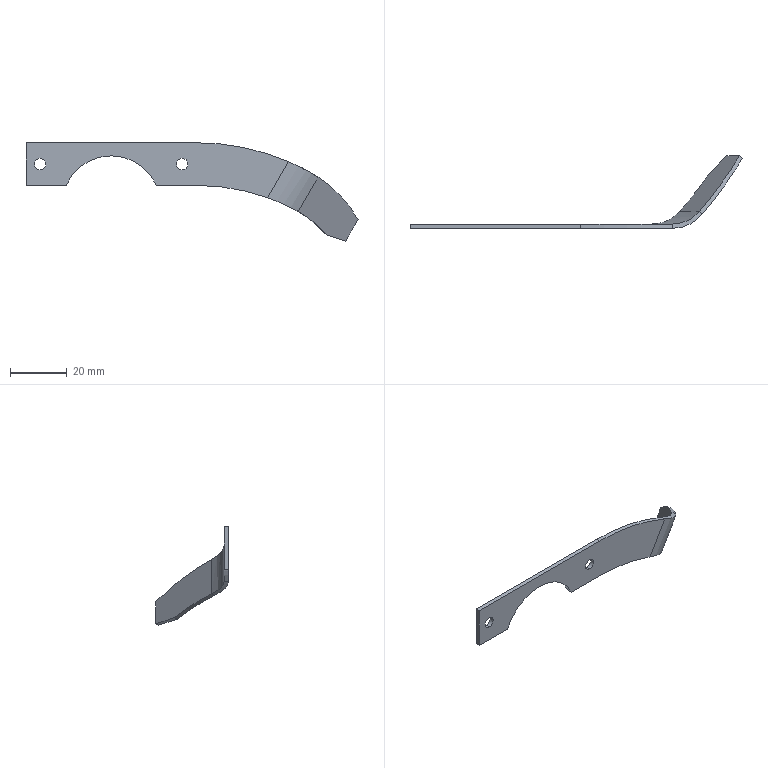Part | SolidWorks | features Chamfer 2, FlatPattern 2, Cut 1, ICE 1, MirrorSolid 1, SM3dBend 1, SMBaseFlange 1, SheetMetal 1 | 1 solid | 24 faces | box 116.818 x 25.618 x 34.656 mm | volume 2408 mm3 | cylinder 12 | plane 10 | spline 2 | commonest cylinder face diameters 4 x4 34.675 x2 148.692 x2 163.932 x2 30 x1 33 x1
STEP:
#1=CARTESIAN_POINT('',(30.,0.,-19.596));
#2=VERTEX_POINT('',#1);
#3=CARTESIAN_POINT('',(14.11,0.,-30.));
#4=VERTEX_POINT('',#3);
#5=CARTESIAN_POINT('',(30.,0.,-36.934));
#6=DIRECTION('',(0.,-1.,0.));
#7=DIRECTION('',(0.,0.,-1.));
#8=AXIS2_PLACEMENT_3D('',#5,#6,#7);
#9=CIRCLE('',#8,17.337);
#10=EDGE_CURVE('',#2,#4,#9,.T.);
#11=ORIENTED_EDGE('',*,*,#10,.F.);
#12=CARTESIAN_POINT('',(30.,-1.5,-19.596));
#13=VERTEX_POINT('',#12);
#14=CARTESIAN_POINT('',(30.,8.5,-19.596));
#15=DIRECTION('',(0.,-1.,0.));
#16=VECTOR('',#15,1000.);
#17=LINE('',#14,#16);
#18=EDGE_CURVE('',#2,#13,#17,.T.);
#19=ORIENTED_EDGE('',*,*,#18,.T.);
#20=CARTESIAN_POINT('',(14.11,-1.5,-30.));
#21=VERTEX_POINT('',#20);
#22=CARTESIAN_POINT('',(30.,-1.5,-36.934));
#23=DIRECTION('',(0.,1.,0.));
#24=DIRECTION('',(0.,0.,1.));
#25=AXIS2_PLACEMENT_3D('',#22,#23,#24);
#26=CIRCLE('',#25,17.337);
#27=EDGE_CURVE('',#21,#13,#26,.T.);
#28=ORIENTED_EDGE('',*,*,#27,.F.);
#29=CARTESIAN_POINT('',(14.11,8.5,-30.));
#30=DIRECTION('',(0.,-1.,0.));
#31=VECTOR('',#30,1000.);
#32=LINE('',#29,#31);
#33=EDGE_CURVE('',#4,#21,#32,.T.);
#34=ORIENTED_EDGE('',*,*,#33,.F.);
#35=EDGE_LOOP('',(#11,#19,#28,#34));
#36=FACE_OUTER_BOUND('',#35,.T.);
#37=CARTESIAN_POINT('',(30.,8.5,-36.934));
#38=DIRECTION('',(0.,-1.,0.));
#39=DIRECTION('',(0.,0.,1.));
#40=AXIS2_PLACEMENT_3D('',#37,#38,#39);
#41=CYLINDRICAL_SURFACE('',#40,17.337);
#42=ADVANCED_FACE('',(#36),#41,.F.);
#43=CARTESIAN_POINT('',(5.,-1.5,-24.5));
#44=VERTEX_POINT('',#43);
#45=CARTESIAN_POINT('',(5.,-1.5,-20.5));
#46=VERTEX_POINT('',#45);
#47=CARTESIAN_POINT('',(5.,-1.5,-22.5));
#48=DIRECTION('',(0.,-1.,0.));
#49=DIRECTION('',(0.,0.,-1.));
#50=AXIS2_PLACEMENT_3D('',#47,#48,#49);
#51=CIRCLE('',#50,2.);
#52=EDGE_CURVE('',#44,#46,#51,.T.);
#53=ORIENTED_EDGE('',*,*,#52,.T.);
#54=CARTESIAN_POINT('',(5.,0.,-20.5));
#55=VERTEX_POINT('',#54);
#56=CARTESIAN_POINT('',(5.,-10.,-20.5));
#57=DIRECTION('',(0.,1.,0.));
#58=VECTOR('',#57,1000.);
#59=LINE('',#56,#58);
#60=EDGE_CURVE('',#46,#55,#59,.T.);
#61=ORIENTED_EDGE('',*,*,#60,.T.);
#62=CARTESIAN_POINT('',(5.,0.,-24.5));
#63=VERTEX_POINT('',#62);
#64=CARTESIAN_POINT('',(5.,0.,-22.5));
#65=DIRECTION('',(0.,-1.,0.));
#66=DIRECTION('',(0.,0.,-1.));
#67=AXIS2_PLACEMENT_3D('',#64,#65,#66);
#68=CIRCLE('',#67,2.);
#69=EDGE_CURVE('',#63,#55,#68,.T.);
#70=ORIENTED_EDGE('',*,*,#69,.F.);
#71=CARTESIAN_POINT('',(5.,-10.,-24.5));
#72=DIRECTION('',(0.,1.,0.));
#73=VECTOR('',#72,1000.);
#74=LINE('',#71,#73);
#75=EDGE_CURVE('',#44,#63,#74,.T.);
#76=ORIENTED_EDGE('',*,*,#75,.F.);
#77=EDGE_LOOP('',(#53,#61,#70,#76));
#78=FACE_OUTER_BOUND('',#77,.T.);
#79=CARTESIAN_POINT('',(5.,-10.,-22.5));
#80=DIRECTION('',(0.,1.,0.));
#81=DIRECTION('',(0.,0.,-1.));
#82=AXIS2_PLACEMENT_3D('',#79,#80,#81);
#83=CYLINDRICAL_SURFACE('',#82,2.);
#84=ADVANCED_FACE('',(#78),#83,.F.);
#85=CARTESIAN_POINT('',(55.,-1.5,-24.5));
#86=VERTEX_POINT('',#85);
#87=CARTESIAN_POINT('',(55.,-1.5,-20.5));
#88=VERTEX_POINT('',#87);
#89=CARTESIAN_POINT('',(55.,-1.5,-22.5));
#90=DIRECTION('',(0.,-1.,0.));
#91=DIRECTION('',(0.,0.,-1.));
#92=AXIS2_PLACEMENT_3D('',#89,#90,#91);
#93=CIRCLE('',#92,2.);
#94=EDGE_CURVE('',#86,#88,#93,.T.);
#95=ORIENTED_EDGE('',*,*,#94,.T.);
#96=CARTESIAN_POINT('',(55.,0.,-20.5));
#97=VERTEX_POINT('',#96);
#98=CARTESIAN_POINT('',(55.,-10.,-20.5));
#99=DIRECTION('',(0.,1.,0.));
#100=VECTOR('',#99,1000.);
#101=LINE('',#98,#100);
#102=EDGE_CURVE('',#88,#97,#101,.T.);
#103=ORIENTED_EDGE('',*,*,#102,.T.);
#104=CARTESIAN_POINT('',(55.,0.,-24.5));
#105=VERTEX_POINT('',#104);
#106=CARTESIAN_POINT('',(55.,0.,-22.5));
#107=DIRECTION('',(0.,-1.,0.));
#108=DIRECTION('',(0.,0.,1.));
#109=AXIS2_PLACEMENT_3D('',#106,#107,#108);
#110=CIRCLE('',#109,2.);
#111=EDGE_CURVE('',#105,#97,#110,.T.);
#112=ORIENTED_EDGE('',*,*,#111,.F.);
#113=CARTESIAN_POINT('',(55.,-10.,-24.5));
#114=DIRECTION('',(0.,1.,0.));
#115=VECTOR('',#114,1000.);
#116=LINE('',#113,#115);
#117=EDGE_CURVE('',#86,#105,#116,.T.);
#118=ORIENTED_EDGE('',*,*,#117,.F.);
#119=EDGE_LOOP('',(#95,#103,#112,#118));
#120=FACE_OUTER_BOUND('',#119,.T.);
#121=CARTESIAN_POINT('',(55.,-10.,-22.5));
#122=DIRECTION('',(0.,1.,0.));
#123=DIRECTION('',(0.,0.,-1.));
#124=AXIS2_PLACEMENT_3D('',#121,#122,#123);
#125=CYLINDRICAL_SURFACE('',#124,2.);
#126=ADVANCED_FACE('',(#120),#125,.F.);
#127=ORIENTED_EDGE('',*,*,#33,.T.);
#128=CARTESIAN_POINT('',(0.,-1.5,-30.));
#129=VERTEX_POINT('',#128);
#130=CARTESIAN_POINT('',(0.,-1.5,-30.));
#131=DIRECTION('',(1.,0.,0.));
#132=VECTOR('',#131,1000.);
#133=LINE('',#130,#132);
#134=EDGE_CURVE('',#129,#21,#133,.T.);
#135=ORIENTED_EDGE('',*,*,#134,.F.);
#136=CARTESIAN_POINT('',(0.,0.,-30.));
#137=VERTEX_POINT('',#136);
#138=CARTESIAN_POINT('',(0.,-1.5,-30.));
#139=DIRECTION('',(0.,1.,0.));
#140=VECTOR('',#139,1000.);
#141=LINE('',#138,#140);
#142=EDGE_CURVE('',#129,#137,#141,.T.);
#143=ORIENTED_EDGE('',*,*,#142,.T.);
#144=CARTESIAN_POINT('',(0.,0.,-30.));
#145=DIRECTION('',(1.,0.,0.));
#146=VECTOR('',#145,1000.);
#147=LINE('',#144,#146);
#148=EDGE_CURVE('',#137,#4,#147,.T.);
#149=ORIENTED_EDGE('',*,*,#148,.T.);
#150=EDGE_LOOP('',(#127,#135,#143,#149));
#151=FACE_OUTER_BOUND('',#150,.T.);
#152=CARTESIAN_POINT('',(0.,-1.5,-30.));
#153=DIRECTION('',(0.,0.,-1.));
#154=DIRECTION('',(1.,0.,0.));
#155=AXIS2_PLACEMENT_3D('',#152,#153,#154);
#156=PLANE('',#155);
#157=ADVANCED_FACE('',(#151),#156,.T.);
#158=CARTESIAN_POINT('',(116.818,22.983,-41.935));
#159=VERTEX_POINT('',#158);
#160=CARTESIAN_POINT('',(112.445,23.057,-49.656));
#161=VERTEX_POINT('',#160);
#162=CARTESIAN_POINT('',(112.315,23.059,-49.886));
#163=DIRECTION('',(-0.4928,0.008327,-0.8701));
#164=VECTOR('',#163,1000.);
#165=LINE('',#162,#164);
#166=EDGE_CURVE('',#159,#161,#165,.T.);
#167=ORIENTED_EDGE('',*,*,#166,.F.);
#168=CARTESIAN_POINT('',(102.727,3.333,-27.041));
#169=VERTEX_POINT('',#168);
#170=CARTESIAN_POINT('',(60.087,1.393,-97.016));
#171=DIRECTION('',(0.6124,-0.7071,-0.3536));
#172=DIRECTION('',(-0.1268,0.3536,-0.9268));
#173=AXIS2_PLACEMENT_3D('',#170,#171,#172);
#174=CIRCLE('',#173,81.966);
#175=EDGE_CURVE('',#159,#169,#174,.T.);
#176=ORIENTED_EDGE('',*,*,#175,.T.);
#177=CARTESIAN_POINT('',(95.741,3.333,-39.141));
#178=VERTEX_POINT('',#177);
#179=CARTESIAN_POINT('',(61.767,3.333,-97.986));
#180=DIRECTION('',(0.5,0.,0.866));
#181=VECTOR('',#180,1000.);
#182=LINE('',#179,#181);
#183=EDGE_CURVE('',#178,#169,#182,.T.);
#184=ORIENTED_EDGE('',*,*,#183,.F.);
#185=CARTESIAN_POINT('',(106.03,16.426,-47.506));
#186=VERTEX_POINT('',#185);
#187=CARTESIAN_POINT('',(59.151,4.003,-103.856));
#188=DIRECTION('',(-0.6124,0.7071,0.3536));
#189=DIRECTION('',(0.1268,-0.3536,0.9268));
#190=AXIS2_PLACEMENT_3D('',#187,#188,#189);
#191=CIRCLE('',#190,74.346);
#192=EDGE_CURVE('',#178,#186,#191,.T.);
#193=ORIENTED_EDGE('',*,*,#192,.T.);
#194=CARTESIAN_POINT('',(106.03,16.426,-47.506));
#195=DIRECTION('',(-0.6772,-0.6999,0.227));
#196=VECTOR('',#195,1000.);
#197=LINE('',#194,#196);
#198=EDGE_CURVE('',#161,#186,#197,.T.);
#199=ORIENTED_EDGE('',*,*,#198,.F.);
#200=EDGE_LOOP('',(#167,#176,#184,#193,#199));
#201=FACE_OUTER_BOUND('',#200,.T.);
#202=CARTESIAN_POINT('',(60.087,1.393,-97.016));
#203=DIRECTION('',(-0.6124,0.7071,0.3536));
#204=DIRECTION('',(-0.1268,0.3536,-0.9268));
#205=AXIS2_PLACEMENT_3D('',#202,#203,#204);
#206=PLANE('',#205);
#207=ADVANCED_FACE('',(#201),#206,.F.);
#208=CARTESIAN_POINT('',(115.899,24.044,-41.405));
#209=VERTEX_POINT('',#208);
#210=CARTESIAN_POINT('',(101.808,4.393,-26.511));
#211=VERTEX_POINT('',#210);
#212=CARTESIAN_POINT('',(59.168,2.454,-96.486));
#213=DIRECTION('',(0.6124,-0.7071,-0.3536));
#214=DIRECTION('',(-0.1268,0.3536,-0.9268));
#215=AXIS2_PLACEMENT_3D('',#212,#213,#214);
#216=CIRCLE('',#215,81.966);
#217=EDGE_CURVE('',#209,#211,#216,.T.);
#218=ORIENTED_EDGE('',*,*,#217,.T.);
#219=CARTESIAN_POINT('',(101.808,4.393,-26.511));
#220=CARTESIAN_POINT('',(102.114,4.04,-26.687));
#221=CARTESIAN_POINT('',(102.421,3.686,-26.864));
#222=CARTESIAN_POINT('',(102.727,3.333,-27.041));
#223=B_SPLINE_CURVE_WITH_KNOTS('',3,(#219,#220,#221,#222),.UNSPECIFIED.,.F.,.F.,(4,4),(0.,1.),.UNSPECIFIED.);
#224=EDGE_CURVE('',#211,#169,#223,.T.);
#225=ORIENTED_EDGE('',*,*,#224,.T.);
#226=ORIENTED_EDGE('',*,*,#175,.F.);
#227=CARTESIAN_POINT('',(116.818,22.983,-41.935));
#228=DIRECTION('',(0.6124,-0.7071,-0.3536));
#229=VECTOR('',#228,1000.);
#230=LINE('',#227,#229);
#231=EDGE_CURVE('',#209,#159,#230,.T.);
#232=ORIENTED_EDGE('',*,*,#231,.F.);
#233=EDGE_LOOP('',(#218,#225,#226,#232));
#234=FACE_OUTER_BOUND('',#233,.T.);
#235=CARTESIAN_POINT('',(60.087,1.393,-97.016));
#236=DIRECTION('',(-0.6124,0.7071,0.3536));
#237=DIRECTION('',(-0.1268,0.3536,-0.9268));
#238=AXIS2_PLACEMENT_3D('',#235,#236,#237);
#239=CYLINDRICAL_SURFACE('',#238,81.966);
#240=ADVANCED_FACE('',(#234),#239,.T.);
#241=ORIENTED_EDGE('',*,*,#192,.F.);
#242=CARTESIAN_POINT('',(94.822,4.393,-38.61));
#243=VERTEX_POINT('',#242);
#244=CARTESIAN_POINT('',(95.741,3.333,-39.141));
#245=CARTESIAN_POINT('',(95.435,3.686,-38.964));
#246=CARTESIAN_POINT('',(95.129,4.04,-38.787));
#247=CARTESIAN_POINT('',(94.822,4.393,-38.61));
#248=B_SPLINE_CURVE_WITH_KNOTS('',3,(#244,#245,#246,#247),.UNSPECIFIED.,.F.,.F.,(4,4),(0.,1.),.UNSPECIFIED.);
#249=EDGE_CURVE('',#178,#243,#248,.T.);
#250=ORIENTED_EDGE('',*,*,#249,.T.);
#251=CARTESIAN_POINT('',(105.112,17.487,-46.976));
#252=VERTEX_POINT('',#251);
#253=CARTESIAN_POINT('',(58.233,5.063,-103.325));
#254=DIRECTION('',(-0.6124,0.7071,0.3536));
#255=DIRECTION('',(0.1268,-0.3536,0.9268));
#256=AXIS2_PLACEMENT_3D('',#253,#254,#255);
#257=CIRCLE('',#256,74.346);
#258=EDGE_CURVE('',#243,#252,#257,.T.);
#259=ORIENTED_EDGE('',*,*,#258,.T.);
#260=CARTESIAN_POINT('',(106.03,16.426,-47.506));
#261=DIRECTION('',(-0.6124,0.7071,0.3536));
#262=VECTOR('',#261,1000.);
#263=LINE('',#260,#262);
#264=EDGE_CURVE('',#186,#252,#263,.T.);
#265=ORIENTED_EDGE('',*,*,#264,.F.);
#266=EDGE_LOOP('',(#241,#250,#259,#265));
#267=FACE_OUTER_BOUND('',#266,.T.);
#268=CARTESIAN_POINT('',(59.151,4.003,-103.856));
#269=DIRECTION('',(-0.6124,0.7071,0.3536));
#270=DIRECTION('',(-0.1268,0.3536,-0.9268));
#271=AXIS2_PLACEMENT_3D('',#268,#269,#270);
#272=CYLINDRICAL_SURFACE('',#271,74.346);
#273=ADVANCED_FACE('',(#267),#272,.F.);
#274=ORIENTED_EDGE('',*,*,#258,.F.);
#275=CARTESIAN_POINT('',(60.848,4.393,-97.456));
#276=DIRECTION('',(0.5,0.,0.866));
#277=VECTOR('',#276,1000.);
#278=LINE('',#275,#277);
#279=EDGE_CURVE('',#243,#211,#278,.T.);
#280=ORIENTED_EDGE('',*,*,#279,.T.);
#281=ORIENTED_EDGE('',*,*,#217,.F.);
#282=CARTESIAN_POINT('',(111.527,24.118,-49.126));
#283=VERTEX_POINT('',#282);
#284=CARTESIAN_POINT('',(78.597,24.674,-107.276));
#285=DIRECTION('',(0.4928,-0.008327,0.8701));
#286=VECTOR('',#285,1000.);
#287=LINE('',#284,#286);
#288=EDGE_CURVE('',#283,#209,#287,.T.);
#289=ORIENTED_EDGE('',*,*,#288,.F.);
#290=CARTESIAN_POINT('',(84.528,-3.789,-40.077));
#291=DIRECTION('',(0.6772,0.6999,-0.227));
#292=VECTOR('',#291,1000.);
#293=LINE('',#290,#292);
#294=EDGE_CURVE('',#252,#283,#293,.T.);
#295=ORIENTED_EDGE('',*,*,#294,.F.);
#296=EDGE_LOOP('',(#274,#280,#281,#289,#295));
#297=FACE_OUTER_BOUND('',#296,.T.);
#298=CARTESIAN_POINT('',(59.168,2.454,-96.486));
#299=DIRECTION('',(-0.6124,0.7071,0.3536));
#300=DIRECTION('',(-0.1268,0.3536,-0.9268));
#301=AXIS2_PLACEMENT_3D('',#298,#299,#300);
#302=PLANE('',#301);
#303=ADVANCED_FACE('',(#297),#302,.T.);
#304=CARTESIAN_POINT('',(60.,0.,-15.));
#305=VERTEX_POINT('',#304);
#306=CARTESIAN_POINT('',(0.,0.,-15.));
#307=VERTEX_POINT('',#306);
#308=CARTESIAN_POINT('',(0.,0.,-15.));
#309=DIRECTION('',(-1.,0.,0.));
#310=VECTOR('',#309,1000.);
#311=LINE('',#308,#310);
#312=EDGE_CURVE('',#305,#307,#311,.T.);
#313=ORIENTED_EDGE('',*,*,#312,.T.);
#314=CARTESIAN_POINT('',(0.,-1.5,-15.));
#315=VERTEX_POINT('',#314);
#316=CARTESIAN_POINT('',(0.,-1.5,-15.));
#317=DIRECTION('',(0.,1.,0.));
#318=VECTOR('',#317,1000.);
#319=LINE('',#316,#318);
#320=EDGE_CURVE('',#315,#307,#319,.T.);
#321=ORIENTED_EDGE('',*,*,#320,.F.);
#322=CARTESIAN_POINT('',(60.,-1.5,-15.));
#323=VERTEX_POINT('',#322);
#324=CARTESIAN_POINT('',(0.,-1.5,-15.));
#325=DIRECTION('',(-1.,0.,0.));
#326=VECTOR('',#325,1000.);
#327=LINE('',#324,#326);
#328=EDGE_CURVE('',#323,#315,#327,.T.);
#329=ORIENTED_EDGE('',*,*,#328,.F.);
#330=CARTESIAN_POINT('',(60.,-1.5,-15.));
#331=DIRECTION('',(0.,1.,0.));
#332=VECTOR('',#331,1000.);
#333=LINE('',#330,#332);
#334=EDGE_CURVE('',#323,#305,#333,.T.);
#335=ORIENTED_EDGE('',*,*,#334,.T.);
#336=EDGE_LOOP('',(#313,#321,#329,#335));
#337=FACE_OUTER_BOUND('',#336,.T.);
#338=CARTESIAN_POINT('',(0.,-1.5,-15.));
#339=DIRECTION('',(0.,0.,1.));
#340=DIRECTION('',(-1.,0.,0.));
#341=AXIS2_PLACEMENT_3D('',#338,#339,#340);
#342=PLANE('',#341);
#343=ADVANCED_FACE('',(#337),#342,.T.);
#344=CARTESIAN_POINT('',(0.,0.,-30.));
#345=DIRECTION('',(0.,0.,-1.));
#346=VECTOR('',#345,1000.);
#347=LINE('',#344,#346);
#348=EDGE_CURVE('',#307,#137,#347,.T.);
#349=ORIENTED_EDGE('',*,*,#348,.T.);
#350=ORIENTED_EDGE('',*,*,#142,.F.);
#351=CARTESIAN_POINT('',(0.,-1.5,-30.));
#352=DIRECTION('',(0.,0.,-1.));
#353=VECTOR('',#352,1000.);
#354=LINE('',#351,#353);
#355=EDGE_CURVE('',#315,#129,#354,.T.);
#356=ORIENTED_EDGE('',*,*,#355,.F.);
#357=ORIENTED_EDGE('',*,*,#320,.T.);
#358=EDGE_LOOP('',(#349,#350,#356,#357));
#359=FACE_OUTER_BOUND('',#358,.T.);
#360=CARTESIAN_POINT('',(0.,-1.5,-30.));
#361=DIRECTION('',(-1.,0.,0.));
#362=DIRECTION('',(0.,0.,-1.));
#363=AXIS2_PLACEMENT_3D('',#360,#361,#362);
#364=PLANE('',#363);
#365=ADVANCED_FACE('',(#359),#364,.T.);
#366=CARTESIAN_POINT('',(45.89,-1.5,-30.));
#367=VERTEX_POINT('',#366);
#368=CARTESIAN_POINT('',(45.89,0.,-30.));
#369=VERTEX_POINT('',#368);
#370=CARTESIAN_POINT('',(45.89,8.5,-30.));
#371=DIRECTION('',(0.,1.,0.));
#372=VECTOR('',#371,1000.);
#373=LINE('',#370,#372);
#374=EDGE_CURVE('',#367,#369,#373,.T.);
#375=ORIENTED_EDGE('',*,*,#374,.T.);
#376=CARTESIAN_POINT('',(60.,0.,-30.));
#377=VERTEX_POINT('',#376);
#378=CARTESIAN_POINT('',(0.,0.,-30.));
#379=DIRECTION('',(1.,0.,0.));
#380=VECTOR('',#379,1000.);
#381=LINE('',#378,#380);
#382=EDGE_CURVE('',#369,#377,#381,.T.);
#383=ORIENTED_EDGE('',*,*,#382,.T.);
#384=CARTESIAN_POINT('',(60.,-1.5,-30.));
#385=VERTEX_POINT('',#384);
#386=CARTESIAN_POINT('',(60.,-1.5,-30.));
#387=DIRECTION('',(0.,1.,0.));
#388=VECTOR('',#387,1000.);
#389=LINE('',#386,#388);
#390=EDGE_CURVE('',#385,#377,#389,.T.);
#391=ORIENTED_EDGE('',*,*,#390,.F.);
#392=CARTESIAN_POINT('',(0.,-1.5,-30.));
#393=DIRECTION('',(1.,0.,0.));
#394=VECTOR('',#393,1000.);
#395=LINE('',#392,#394);
#396=EDGE_CURVE('',#367,#385,#395,.T.);
#397=ORIENTED_EDGE('',*,*,#396,.F.);
#398=EDGE_LOOP('',(#375,#383,#391,#397));
#399=FACE_OUTER_BOUND('',#398,.T.);
#400=CARTESIAN_POINT('',(0.,-1.5,-30.));
#401=DIRECTION('',(0.,0.,-1.));
#402=DIRECTION('',(1.,0.,0.));
#403=AXIS2_PLACEMENT_3D('',#400,#401,#402);
#404=PLANE('',#403);
#405=ADVANCED_FACE('',(#399),#404,.T.);
#406=ORIENTED_EDGE('',*,*,#52,.F.);
#407=CARTESIAN_POINT('',(5.,-1.5,-22.5));
#408=DIRECTION('',(0.,-1.,0.));
#409=DIRECTION('',(0.,0.,-1.));
#410=AXIS2_PLACEMENT_3D('',#407,#408,#409);
#411=CIRCLE('',#410,2.);
#412=EDGE_CURVE('',#46,#44,#411,.T.);
#413=ORIENTED_EDGE('',*,*,#412,.F.);
#414=EDGE_LOOP('',(#406,#413));
#415=FACE_BOUND('',#414,.T.);
#416=ORIENTED_EDGE('',*,*,#94,.F.);
#417=CARTESIAN_POINT('',(55.,-1.5,-22.5));
#418=DIRECTION('',(0.,-1.,0.));
#419=DIRECTION('',(0.,0.,-1.));
#420=AXIS2_PLACEMENT_3D('',#417,#418,#419);
#421=CIRCLE('',#420,2.);
#422=EDGE_CURVE('',#88,#86,#421,.T.);
#423=ORIENTED_EDGE('',*,*,#422,.F.);
#424=EDGE_LOOP('',(#416,#423));
#425=FACE_BOUND('',#424,.T.);
#426=ORIENTED_EDGE('',*,*,#396,.T.);
#427=CARTESIAN_POINT('',(85.039,-1.5,-34.343));
#428=VERTEX_POINT('',#427);
#429=CARTESIAN_POINT('',(60.,-1.5,-104.346));
#430=DIRECTION('',(0.,1.,0.));
#431=DIRECTION('',(0.,0.,1.));
#432=AXIS2_PLACEMENT_3D('',#429,#430,#431);
#433=CIRCLE('',#432,74.346);
#434=EDGE_CURVE('',#385,#428,#433,.T.);
#435=ORIENTED_EDGE('',*,*,#434,.T.);
#436=CARTESIAN_POINT('',(92.362,-1.5,-21.659));
#437=VERTEX_POINT('',#436);
#438=CARTESIAN_POINT('',(51.662,-1.5,-92.152));
#439=DIRECTION('',(0.5,0.,0.866));
#440=VECTOR('',#439,1000.);
#441=LINE('',#438,#440);
#442=EDGE_CURVE('',#428,#437,#441,.T.);
#443=ORIENTED_EDGE('',*,*,#442,.T.);
#444=CARTESIAN_POINT('',(60.,-1.5,-96.966));
#445=DIRECTION('',(0.,-1.,0.));
#446=DIRECTION('',(0.,0.,-1.));
#447=AXIS2_PLACEMENT_3D('',#444,#445,#446);
#448=CIRCLE('',#447,81.966);
#449=EDGE_CURVE('',#437,#323,#448,.T.);
#450=ORIENTED_EDGE('',*,*,#449,.T.);
#451=ORIENTED_EDGE('',*,*,#328,.T.);
#452=ORIENTED_EDGE('',*,*,#355,.T.);
#453=ORIENTED_EDGE('',*,*,#134,.T.);
#454=ORIENTED_EDGE('',*,*,#27,.T.);
#455=CARTESIAN_POINT('',(30.,-1.5,-36.934));
#456=DIRECTION('',(0.,1.,0.));
#457=DIRECTION('',(0.,0.,1.));
#458=AXIS2_PLACEMENT_3D('',#455,#456,#457);
#459=CIRCLE('',#458,17.337);
#460=EDGE_CURVE('',#13,#367,#459,.T.);
#461=ORIENTED_EDGE('',*,*,#460,.T.);
#462=EDGE_LOOP('',(#426,#435,#443,#450,#451,#452,#453,#454,#461));
#463=FACE_OUTER_BOUND('',#462,.T.);
#464=CARTESIAN_POINT('',(60.,-1.5,-96.966));
#465=DIRECTION('',(0.,1.,0.));
#466=DIRECTION('',(0.,0.,-1.));
#467=AXIS2_PLACEMENT_3D('',#464,#465,#466);
#468=PLANE('',#467);
#469=ADVANCED_FACE('',(#415,#425,#463),#468,.F.);
#470=ORIENTED_EDGE('',*,*,#434,.F.);
#471=ORIENTED_EDGE('',*,*,#390,.T.);
#472=CARTESIAN_POINT('',(85.039,0.,-34.343));
#473=VERTEX_POINT('',#472);
#474=CARTESIAN_POINT('',(60.,0.,-104.346));
#475=DIRECTION('',(0.,1.,0.));
#476=DIRECTION('',(0.,0.,1.));
#477=AXIS2_PLACEMENT_3D('',#474,#475,#476);
#478=CIRCLE('',#477,74.346);
#479=EDGE_CURVE('',#377,#473,#478,.T.);
#480=ORIENTED_EDGE('',*,*,#479,.T.);
#481=CARTESIAN_POINT('',(85.039,-1.5,-34.343));
#482=CARTESIAN_POINT('',(85.039,0.,-34.343));
#483=B_SPLINE_CURVE_WITH_KNOTS('',1,(#481,#482),.UNSPECIFIED.,.F.,.F.,(2,2),(0.,1.),.UNSPECIFIED.);
#484=EDGE_CURVE('',#428,#473,#483,.T.);
#485=ORIENTED_EDGE('',*,*,#484,.F.);
#486=EDGE_LOOP('',(#470,#471,#480,#485));
#487=FACE_OUTER_BOUND('',#486,.T.);
#488=CARTESIAN_POINT('',(60.,-1.5,-104.346));
#489=DIRECTION('',(0.,1.,0.));
#490=DIRECTION('',(0.,0.,-1.));
#491=AXIS2_PLACEMENT_3D('',#488,#489,#490);
#492=CYLINDRICAL_SURFACE('',#491,74.346);
#493=ADVANCED_FACE('',(#487),#492,.F.);
#494=CARTESIAN_POINT('',(30.,0.,-36.934));
#495=DIRECTION('',(0.,-1.,0.));
#496=DIRECTION('',(0.,0.,-1.));
#497=AXIS2_PLACEMENT_3D('',#494,#495,#496);
#498=CIRCLE('',#497,17.337);
#499=EDGE_CURVE('',#369,#2,#498,.T.);
#500=ORIENTED_EDGE('',*,*,#499,.T.);
#501=ORIENTED_EDGE('',*,*,#10,.T.);
#502=ORIENTED_EDGE('',*,*,#148,.F.);
#503=ORIENTED_EDGE('',*,*,#348,.F.);
#504=ORIENTED_EDGE('',*,*,#312,.F.);
#505=CARTESIAN_POINT('',(92.362,0.,-21.659));
#506=VERTEX_POINT('',#505);
#507=CARTESIAN_POINT('',(60.,0.,-96.966));
#508=DIRECTION('',(0.,-1.,0.));
#509=DIRECTION('',(0.,0.,-1.));
#510=AXIS2_PLACEMENT_3D('',#507,#508,#509);
#511=CIRCLE('',#510,81.966);
#512=EDGE_CURVE('',#506,#305,#511,.T.);
#513=ORIENTED_EDGE('',*,*,#512,.F.);
#514=CARTESIAN_POINT('',(51.662,0.,-92.152));
#515=DIRECTION('',(0.5,0.,0.866));
#516=VECTOR('',#515,1000.);
#517=LINE('',#514,#516);
#518=EDGE_CURVE('',#473,#506,#517,.T.);
#519=ORIENTED_EDGE('',*,*,#518,.F.);
#520=ORIENTED_EDGE('',*,*,#479,.F.);
#521=ORIENTED_EDGE('',*,*,#382,.F.);
#522=EDGE_LOOP('',(#500,#501,#502,#503,#504,#513,#519,#520,#521));
#523=FACE_OUTER_BOUND('',#522,.T.);
#524=ORIENTED_EDGE('',*,*,#69,.T.);
#525=CARTESIAN_POINT('',(5.,0.,-22.5));
#526=DIRECTION('',(0.,-1.,0.));
#527=DIRECTION('',(0.,0.,-1.));
#528=AXIS2_PLACEMENT_3D('',#525,#526,#527);
#529=CIRCLE('',#528,2.);
#530=EDGE_CURVE('',#55,#63,#529,.T.);
#531=ORIENTED_EDGE('',*,*,#530,.T.);
#532=EDGE_LOOP('',(#524,#531));
#533=FACE_BOUND('',#532,.T.);
#534=ORIENTED_EDGE('',*,*,#111,.T.);
#535=CARTESIAN_POINT('',(55.,0.,-22.5));
#536=DIRECTION('',(0.,-1.,0.));
#537=DIRECTION('',(0.,0.,1.));
#538=AXIS2_PLACEMENT_3D('',#535,#536,#537);
#539=CIRCLE('',#538,2.);
#540=EDGE_CURVE('',#97,#105,#539,.T.);
#541=ORIENTED_EDGE('',*,*,#540,.T.);
#542=EDGE_LOOP('',(#534,#541));
#543=FACE_BOUND('',#542,.T.);
#544=CARTESIAN_POINT('',(60.,0.,-96.966));
#545=DIRECTION('',(0.,1.,0.));
#546=DIRECTION('',(0.,0.,-1.));
#547=AXIS2_PLACEMENT_3D('',#544,#545,#546);
#548=PLANE('',#547);
#549=ADVANCED_FACE('',(#523,#533,#543),#548,.T.);
#550=ORIENTED_EDGE('',*,*,#512,.T.);
#551=ORIENTED_EDGE('',*,*,#334,.F.);
#552=ORIENTED_EDGE('',*,*,#449,.F.);
#553=CARTESIAN_POINT('',(92.362,0.,-21.659));
#554=CARTESIAN_POINT('',(92.362,-1.5,-21.659));
#555=B_SPLINE_CURVE_WITH_KNOTS('',1,(#553,#554),.UNSPECIFIED.,.F.,.F.,(2,2),(0.,1.),.UNSPECIFIED.);
#556=EDGE_CURVE('',#506,#437,#555,.T.);
#557=ORIENTED_EDGE('',*,*,#556,.F.);
#558=EDGE_LOOP('',(#550,#551,#552,#557));
#559=FACE_OUTER_BOUND('',#558,.T.);
#560=CARTESIAN_POINT('',(60.,-1.5,-96.966));
#561=DIRECTION('',(0.,1.,0.));
#562=DIRECTION('',(0.,0.,-1.));
#563=AXIS2_PLACEMENT_3D('',#560,#561,#562);
#564=CYLINDRICAL_SURFACE('',#563,81.966);
#565=ADVANCED_FACE('',(#559),#564,.T.);
#566=ORIENTED_EDGE('',*,*,#249,.F.);
#567=CARTESIAN_POINT('',(95.741,3.333,-39.141));
#568=CARTESIAN_POINT('',(94.963,2.448,-38.718));
#569=CARTESIAN_POINT('',(94.143,1.724,-38.291));
#570=CARTESIAN_POINT('',(92.918,0.8426,-37.68));
#571=CARTESIAN_POINT('',(92.51,0.5825,-37.482));
#572=CARTESIAN_POINT('',(91.906,0.237,-37.195));
#573=CARTESIAN_POINT('',(91.706,0.1293,-37.102));
#574=CARTESIAN_POINT('',(91.408,-0.02187,-36.965));
#575=CARTESIAN_POINT('',(91.309,-0.07052,-36.919));
#576=CARTESIAN_POINT('',(91.162,-0.141,-36.853));
#577=CARTESIAN_POINT('',(91.113,-0.1641,-36.83));
#578=CARTESIAN_POINT('',(91.04,-0.1981,-36.797));
#579=CARTESIAN_POINT('',(91.015,-0.2093,-36.786));
#580=CARTESIAN_POINT('',(90.979,-0.226,-36.77));
#581=CARTESIAN_POINT('',(90.966,-0.2315,-36.765));
#582=CARTESIAN_POINT('',(90.948,-0.2398,-36.756));
#583=CARTESIAN_POINT('',(90.942,-0.2426,-36.754));
#584=CARTESIAN_POINT('',(90.93,-0.2481,-36.748));
#585=CARTESIAN_POINT('',(90.923,-0.2513,-36.745));
#586=CARTESIAN_POINT('',(90.29,-0.5353,-36.463));
#587=CARTESIAN_POINT('',(89.493,-0.8384,-36.126));
#588=CARTESIAN_POINT('',(87.533,-1.321,-35.327));
#589=CARTESIAN_POINT('',(86.371,-1.5,-34.863));
#590=CARTESIAN_POINT('',(85.039,-1.5,-34.343));
#591=B_SPLINE_CURVE_WITH_KNOTS('',3,(#567,#568,#569,#570,#571,#572,#573,#574,#575,#576,#577,#578,#579,#580,#581,#582,#583,#584,#585,#586,#587,#588,#589,#590),.UNSPECIFIED.,.F.,.F.,(4,2,2,2,2,2,2,2,2,2,2,4),(0.,0.25,0.375,0.4375,0.4688,0.4844,0.4922,0.4961,0.498,0.5,0.75,1.),.UNSPECIFIED.);
#592=EDGE_CURVE('',#178,#428,#591,.T.);
#593=ORIENTED_EDGE('',*,*,#592,.T.);
#594=ORIENTED_EDGE('',*,*,#484,.T.);
#595=CARTESIAN_POINT('',(94.822,4.393,-38.61));
#596=CARTESIAN_POINT('',(94.114,3.589,-38.229));
#597=CARTESIAN_POINT('',(93.367,2.931,-37.843));
#598=CARTESIAN_POINT('',(92.249,2.13,-37.294));
#599=CARTESIAN_POINT('',(91.877,1.893,-37.116));
#600=CARTESIAN_POINT('',(91.325,1.579,-36.86));
#601=CARTESIAN_POINT('',(91.143,1.481,-36.777));
#602=CARTESIAN_POINT('',(90.871,1.344,-36.654));
#603=CARTESIAN_POINT('',(90.735,1.277,-36.594));
#604=CARTESIAN_POINT('',(90.579,1.204,-36.525));
#605=CARTESIAN_POINT('',(90.5,1.168,-36.491));
#606=CARTESIAN_POINT('',(90.461,1.151,-36.474));
#607=CARTESIAN_POINT('',(90.445,1.143,-36.466));
#608=CARTESIAN_POINT('',(90.434,1.138,-36.462));
#609=CARTESIAN_POINT('',(90.427,1.135,-36.459));
#610=CARTESIAN_POINT('',(89.849,0.877,-36.208));
#611=CARTESIAN_POINT('',(89.119,0.6015,-35.91));
#612=CARTESIAN_POINT('',(87.325,0.1628,-35.206));
#613=CARTESIAN_POINT('',(86.259,0.,-34.798));
#614=CARTESIAN_POINT('',(85.039,0.,-34.343));
#615=B_SPLINE_CURVE_WITH_KNOTS('',3,(#595,#596,#597,#598,#599,#600,#601,#602,#603,#604,#605,#606,#607,#608,#609,#610,#611,#612,#613,#614),.UNSPECIFIED.,.F.,.F.,(4,2,2,2,1,1,1,1,2,2,2,4),(0.,0.25,0.375,0.4375,0.4688,0.4844,0.4922,0.4961,0.498,0.5,0.75,1.),.UNSPECIFIED.);
#616=EDGE_CURVE('',#243,#473,#615,.T.);
#617=ORIENTED_EDGE('',*,*,#616,.F.);
#618=EDGE_LOOP('',(#566,#593,#594,#617));
#619=FACE_OUTER_BOUND('',#618,.T.);
#620=CARTESIAN_POINT('',(95.741,3.333,-39.141));
#621=CARTESIAN_POINT('',(94.963,2.448,-38.718));
#622=CARTESIAN_POINT('',(94.143,1.724,-38.291));
#623=CARTESIAN_POINT('',(92.918,0.8426,-37.68));
#624=CARTESIAN_POINT('',(92.51,0.5825,-37.482));
#625=CARTESIAN_POINT('',(91.906,0.237,-37.195));
#626=CARTESIAN_POINT('',(91.706,0.1293,-37.102));
#627=CARTESIAN_POINT('',(91.408,-0.02187,-36.965));
#628=CARTESIAN_POINT('',(91.309,-0.07052,-36.919));
#629=CARTESIAN_POINT('',(91.162,-0.141,-36.853));
#630=CARTESIAN_POINT('',(91.113,-0.1641,-36.83));
#631=CARTESIAN_POINT('',(91.04,-0.1981,-36.797));
#632=CARTESIAN_POINT('',(91.015,-0.2093,-36.786));
#633=CARTESIAN_POINT('',(90.979,-0.226,-36.77));
#634=CARTESIAN_POINT('',(90.966,-0.2315,-36.765));
#635=CARTESIAN_POINT('',(90.948,-0.2398,-36.756));
#636=CARTESIAN_POINT('',(90.942,-0.2426,-36.754));
#637=CARTESIAN_POINT('',(90.93,-0.2481,-36.748));
#638=CARTESIAN_POINT('',(90.923,-0.2513,-36.745));
#639=CARTESIAN_POINT('',(90.29,-0.5353,-36.463));
#640=CARTESIAN_POINT('',(89.493,-0.8384,-36.126));
#641=CARTESIAN_POINT('',(87.533,-1.321,-35.327));
#642=CARTESIAN_POINT('',(86.371,-1.5,-34.863));
#643=CARTESIAN_POINT('',(85.039,-1.5,-34.343));
#644=CARTESIAN_POINT('',(94.822,4.393,-38.61));
#645=CARTESIAN_POINT('',(94.114,3.589,-38.228));
#646=CARTESIAN_POINT('',(93.367,2.931,-37.843));
#647=CARTESIAN_POINT('',(92.249,2.13,-37.294));
#648=CARTESIAN_POINT('',(91.877,1.893,-37.116));
#649=CARTESIAN_POINT('',(91.325,1.579,-36.86));
#650=CARTESIAN_POINT('',(91.143,1.481,-36.777));
#651=CARTESIAN_POINT('',(90.871,1.344,-36.654));
#652=CARTESIAN_POINT('',(90.781,1.3,-36.614));
#653=CARTESIAN_POINT('',(90.646,1.235,-36.554));
#654=CARTESIAN_POINT('',(90.601,1.214,-36.535));
#655=CARTESIAN_POINT('',(90.534,1.184,-36.505));
#656=CARTESIAN_POINT('',(90.512,1.173,-36.496));
#657=CARTESIAN_POINT('',(90.478,1.158,-36.481));
#658=CARTESIAN_POINT('',(90.467,1.153,-36.476));
#659=CARTESIAN_POINT('',(90.45,1.146,-36.469));
#660=CARTESIAN_POINT('',(90.445,1.143,-36.466));
#661=CARTESIAN_POINT('',(90.434,1.138,-36.462));
#662=CARTESIAN_POINT('',(90.427,1.135,-36.459));
#663=CARTESIAN_POINT('',(89.849,0.877,-36.208));
#664=CARTESIAN_POINT('',(89.119,0.6015,-35.91));
#665=CARTESIAN_POINT('',(87.325,0.1628,-35.206));
#666=CARTESIAN_POINT('',(86.26,0.,-34.799));
#667=CARTESIAN_POINT('',(85.039,0.,-34.343));
#668=B_SPLINE_SURFACE_WITH_KNOTS('',1,3,((#620,#621,#622,#623,#624,#625,#626,#627,#628,#629,#630,#631,#632,#633,#634,#635,#636,#637,#638,#639,#640,#641,#642,#643),(#644,#645,#646,#647,#648,#649,#650,#651,#652,#653,#654,#655,#656,#657,#658,#659,#660,#661,#662,#663,#664,#665,#666,#667)),.UNSPECIFIED.,.F.,.F.,.F.,(2,2),(4,2,2,2,2,2,2,2,2,2,2,4),(0.,1.),(0.,0.25,0.375,0.4375,0.4688,0.4844,0.4922,0.4961,0.498,0.5,0.75,1.),.UNSPECIFIED.);
#669=ADVANCED_FACE('',(#619),#668,.F.);
#670=ORIENTED_EDGE('',*,*,#556,.T.);
#671=CARTESIAN_POINT('',(92.362,-1.5,-21.659));
#672=CARTESIAN_POINT('',(93.46,-1.5,-22.142));
#673=CARTESIAN_POINT('',(94.494,-1.371,-22.617));
#674=CARTESIAN_POINT('',(95.928,-1.039,-23.301));
#675=CARTESIAN_POINT('',(96.386,-0.9058,-23.525));
#676=CARTESIAN_POINT('',(97.041,-0.678,-23.852));
#677=CARTESIAN_POINT('',(97.255,-0.5975,-23.96));
#678=CARTESIAN_POINT('',(97.567,-0.4706,-24.12));
#679=CARTESIAN_POINT('',(97.67,-0.4273,-24.173));
#680=CARTESIAN_POINT('',(97.822,-0.3609,-24.251));
#681=CARTESIAN_POINT('',(97.872,-0.3385,-24.278));
#682=CARTESIAN_POINT('',(97.947,-0.3046,-24.317));
#683=CARTESIAN_POINT('',(97.972,-0.2933,-24.33));
#684=CARTESIAN_POINT('',(98.009,-0.2761,-24.349));
#685=CARTESIAN_POINT('',(98.022,-0.2704,-24.356));
#686=CARTESIAN_POINT('',(98.04,-0.2618,-24.366));
#687=CARTESIAN_POINT('',(98.047,-0.259,-24.369));
#688=CARTESIAN_POINT('',(98.056,-0.2546,-24.374));
#689=CARTESIAN_POINT('',(98.059,-0.2532,-24.375));
#690=CARTESIAN_POINT('',(98.065,-0.2503,-24.379));
#691=CARTESIAN_POINT('',(98.069,-0.2485,-24.381));
#692=CARTESIAN_POINT('',(98.663,0.0289,-24.693));
#693=CARTESIAN_POINT('',(99.38,0.4161,-25.089));
#694=CARTESIAN_POINT('',(100.975,1.558,-26.));
#695=CARTESIAN_POINT('',(101.853,2.314,-26.516));
#696=CARTESIAN_POINT('',(102.727,3.333,-27.041));
#697=B_SPLINE_CURVE_WITH_KNOTS('',3,(#671,#672,#673,#674,#675,#676,#677,#678,#679,#680,#681,#682,#683,#684,#685,#686,#687,#688,#689,#690,#691,#692,#693,#694,#695,#696),.UNSPECIFIED.,.F.,.F.,(4,2,2,2,2,2,2,2,2,2,2,2,4),(0.,0.25,0.375,0.4375,0.4688,0.4844,0.4922,0.4961,0.498,0.499,0.5,0.75,1.),.UNSPECIFIED.);
#698=EDGE_CURVE('',#437,#169,#697,.T.);
#699=ORIENTED_EDGE('',*,*,#698,.T.);
#700=ORIENTED_EDGE('',*,*,#224,.F.);
#701=CARTESIAN_POINT('',(92.362,0.,-21.659));
#702=CARTESIAN_POINT('',(93.365,0.,-22.088));
#703=CARTESIAN_POINT('',(94.311,0.1174,-22.511));
#704=CARTESIAN_POINT('',(95.62,0.4188,-23.123));
#705=CARTESIAN_POINT('',(96.038,0.5401,-23.324));
#706=CARTESIAN_POINT('',(96.636,0.7472,-23.618));
#707=CARTESIAN_POINT('',(96.831,0.8205,-23.715));
#708=CARTESIAN_POINT('',(97.115,0.9358,-23.859));
#709=CARTESIAN_POINT('',(97.256,0.9949,-23.93));
#710=CARTESIAN_POINT('',(97.416,1.066,-24.013));
#711=CARTESIAN_POINT('',(97.496,1.102,-24.054));
#712=CARTESIAN_POINT('',(97.535,1.12,-24.075));
#713=CARTESIAN_POINT('',(97.552,1.128,-24.083));
#714=CARTESIAN_POINT('',(97.564,1.133,-24.089));
#715=CARTESIAN_POINT('',(97.571,1.137,-24.093));
#716=CARTESIAN_POINT('',(98.114,1.39,-24.376));
#717=CARTESIAN_POINT('',(98.767,1.742,-24.735));
#718=CARTESIAN_POINT('',(100.217,2.78,-25.563));
#719=CARTESIAN_POINT('',(101.016,3.468,-26.032));
#720=CARTESIAN_POINT('',(101.808,4.393,-26.511));
#721=B_SPLINE_CURVE_WITH_KNOTS('',3,(#701,#702,#703,#704,#705,#706,#707,#708,#709,#710,#711,#712,#713,#714,#715,#716,#717,#718,#719,#720),.UNSPECIFIED.,.F.,.F.,(4,2,2,2,1,1,1,1,2,2,2,4),(0.,0.25,0.375,0.4375,0.4687,0.4844,0.4922,0.4961,0.498,0.5,0.75,1.),.UNSPECIFIED.);
#722=EDGE_CURVE('',#506,#211,#721,.T.);
#723=ORIENTED_EDGE('',*,*,#722,.F.);
#724=EDGE_LOOP('',(#670,#699,#700,#723));
#725=FACE_OUTER_BOUND('',#724,.T.);
#726=CARTESIAN_POINT('',(92.362,-1.5,-21.659));
#727=CARTESIAN_POINT('',(93.46,-1.5,-22.142));
#728=CARTESIAN_POINT('',(94.494,-1.371,-22.617));
#729=CARTESIAN_POINT('',(95.928,-1.039,-23.301));
#730=CARTESIAN_POINT('',(96.386,-0.9058,-23.525));
#731=CARTESIAN_POINT('',(97.041,-0.678,-23.852));
#732=CARTESIAN_POINT('',(97.255,-0.5975,-23.96));
#733=CARTESIAN_POINT('',(97.567,-0.4706,-24.12));
#734=CARTESIAN_POINT('',(97.67,-0.4273,-24.173));
#735=CARTESIAN_POINT('',(97.822,-0.3609,-24.251));
#736=CARTESIAN_POINT('',(97.872,-0.3385,-24.278));
#737=CARTESIAN_POINT('',(97.947,-0.3046,-24.317));
#738=CARTESIAN_POINT('',(97.972,-0.2933,-24.33));
#739=CARTESIAN_POINT('',(98.009,-0.2761,-24.349));
#740=CARTESIAN_POINT('',(98.022,-0.2704,-24.356));
#741=CARTESIAN_POINT('',(98.04,-0.2618,-24.366));
#742=CARTESIAN_POINT('',(98.047,-0.259,-24.369));
#743=CARTESIAN_POINT('',(98.056,-0.2546,-24.374));
#744=CARTESIAN_POINT('',(98.059,-0.2532,-24.375));
#745=CARTESIAN_POINT('',(98.065,-0.2503,-24.379));
#746=CARTESIAN_POINT('',(98.069,-0.2485,-24.381));
#747=CARTESIAN_POINT('',(98.663,0.0289,-24.693));
#748=CARTESIAN_POINT('',(99.38,0.4161,-25.089));
#749=CARTESIAN_POINT('',(100.975,1.558,-26.));
#750=CARTESIAN_POINT('',(101.853,2.314,-26.516));
#751=CARTESIAN_POINT('',(102.727,3.333,-27.041));
#752=CARTESIAN_POINT('',(92.362,0.,-21.659));
#753=CARTESIAN_POINT('',(93.366,0.,-22.088));
#754=CARTESIAN_POINT('',(94.311,0.1174,-22.511));
#755=CARTESIAN_POINT('',(95.62,0.4188,-23.123));
#756=CARTESIAN_POINT('',(96.038,0.5401,-23.324));
#757=CARTESIAN_POINT('',(96.636,0.7472,-23.618));
#758=CARTESIAN_POINT('',(96.831,0.8205,-23.715));
#759=CARTESIAN_POINT('',(97.115,0.9358,-23.859));
#760=CARTESIAN_POINT('',(97.209,0.9752,-23.906));
#761=CARTESIAN_POINT('',(97.348,1.036,-23.978));
#762=CARTESIAN_POINT('',(97.393,1.056,-24.001));
#763=CARTESIAN_POINT('',(97.462,1.087,-24.036));
#764=CARTESIAN_POINT('',(97.485,1.097,-24.048));
#765=CARTESIAN_POINT('',(97.518,1.113,-24.066));
#766=CARTESIAN_POINT('',(97.53,1.118,-24.072));
#767=CARTESIAN_POINT('',(97.547,1.126,-24.081));
#768=CARTESIAN_POINT('',(97.552,1.128,-24.083));
#769=CARTESIAN_POINT('',(97.561,1.132,-24.088));
#770=CARTESIAN_POINT('',(97.564,1.133,-24.089));
#771=CARTESIAN_POINT('',(97.569,1.136,-24.092));
#772=CARTESIAN_POINT('',(97.573,1.138,-24.094));
#773=CARTESIAN_POINT('',(98.114,1.39,-24.376));
#774=CARTESIAN_POINT('',(98.767,1.742,-24.735));
#775=CARTESIAN_POINT('',(100.217,2.78,-25.563));
#776=CARTESIAN_POINT('',(101.015,3.467,-26.032));
#777=CARTESIAN_POINT('',(101.808,4.393,-26.511));
#778=B_SPLINE_SURFACE_WITH_KNOTS('',1,3,((#726,#727,#728,#729,#730,#731,#732,#733,#734,#735,#736,#737,#738,#739,#740,#741,#742,#743,#744,#745,#746,#747,#748,#749,#750,#751),(#752,#753,#754,#755,#756,#757,#758,#759,#760,#761,#762,#763,#764,#765,#766,#767,#768,#769,#770,#771,#772,#773,#774,#775,#776,#777)),.UNSPECIFIED.,.F.,.F.,.F.,(2,2),(4,2,2,2,2,2,2,2,2,2,2,2,4),(0.,1.),(0.,0.25,0.375,0.4375,0.4688,0.4844,0.4922,0.4961,0.498,0.499,0.5,0.75,1.),.UNSPECIFIED.);
#779=ADVANCED_FACE('',(#725),#778,.F.);
#780=ORIENTED_EDGE('',*,*,#698,.F.);
#781=ORIENTED_EDGE('',*,*,#442,.F.);
#782=ORIENTED_EDGE('',*,*,#592,.F.);
#783=ORIENTED_EDGE('',*,*,#183,.T.);
#784=EDGE_LOOP('',(#780,#781,#782,#783));
#785=FACE_OUTER_BOUND('',#784,.T.);
#786=CARTESIAN_POINT('',(101.497,15.,-5.836));
#787=DIRECTION('',(-0.5,0.,-0.866));
#788=DIRECTION('',(0.866,0.,-0.5));
#789=AXIS2_PLACEMENT_3D('',#786,#787,#788);
#790=CYLINDRICAL_SURFACE('',#789,16.5);
#791=ADVANCED_FACE('',(#785),#790,.T.);
#792=ORIENTED_EDGE('',*,*,#722,.T.);
#793=ORIENTED_EDGE('',*,*,#279,.F.);
#794=ORIENTED_EDGE('',*,*,#616,.T.);
#795=ORIENTED_EDGE('',*,*,#518,.T.);
#796=EDGE_LOOP('',(#792,#793,#794,#795));
#797=FACE_OUTER_BOUND('',#796,.T.);
#798=CARTESIAN_POINT('',(101.497,15.,-5.836));
#799=DIRECTION('',(-0.5,0.,-0.866));
#800=DIRECTION('',(0.866,0.,-0.5));
#801=AXIS2_PLACEMENT_3D('',#798,#799,#800);
#802=CYLINDRICAL_SURFACE('',#801,15.);
#803=ADVANCED_FACE('',(#797),#802,.F.);
#804=ORIENTED_EDGE('',*,*,#288,.T.);
#805=ORIENTED_EDGE('',*,*,#231,.T.);
#806=ORIENTED_EDGE('',*,*,#166,.T.);
#807=CARTESIAN_POINT('',(112.445,23.057,-49.656));
#808=DIRECTION('',(0.6124,-0.7071,-0.3536));
#809=VECTOR('',#808,1000.);
#810=LINE('',#807,#809);
#811=EDGE_CURVE('',#283,#161,#810,.T.);
#812=ORIENTED_EDGE('',*,*,#811,.F.);
#813=EDGE_LOOP('',(#804,#805,#806,#812));
#814=FACE_OUTER_BOUND('',#813,.T.);
#815=CARTESIAN_POINT('',(112.315,23.059,-49.886));
#816=DIRECTION('',(-0.6182,-0.7071,0.3433));
#817=DIRECTION('',(-0.6124,0.7071,0.3536));
#818=AXIS2_PLACEMENT_3D('',#815,#816,#817);
#819=PLANE('',#818);
#820=ADVANCED_FACE('',(#814),#819,.F.);
#821=ORIENTED_EDGE('',*,*,#198,.T.);
#822=ORIENTED_EDGE('',*,*,#264,.T.);
#823=ORIENTED_EDGE('',*,*,#294,.T.);
#824=ORIENTED_EDGE('',*,*,#811,.T.);
#825=EDGE_LOOP('',(#821,#822,#823,#824));
#826=FACE_OUTER_BOUND('',#825,.T.);
#827=CARTESIAN_POINT('',(106.03,16.426,-47.506));
#828=DIRECTION('',(0.408,-0.1004,0.9075));
#829=DIRECTION('',(-0.6124,0.7071,0.3536));
#830=AXIS2_PLACEMENT_3D('',#827,#828,#829);
#831=PLANE('',#830);
#832=ADVANCED_FACE('',(#826),#831,.F.);
#833=ORIENTED_EDGE('',*,*,#102,.F.);
#834=ORIENTED_EDGE('',*,*,#422,.T.);
#835=ORIENTED_EDGE('',*,*,#117,.T.);
#836=ORIENTED_EDGE('',*,*,#540,.F.);
#837=EDGE_LOOP('',(#833,#834,#835,#836));
#838=FACE_OUTER_BOUND('',#837,.T.);
#839=CARTESIAN_POINT('',(55.,-10.,-22.5));
#840=DIRECTION('',(0.,1.,0.));
#841=DIRECTION('',(0.,0.,-1.));
#842=AXIS2_PLACEMENT_3D('',#839,#840,#841);
#843=CYLINDRICAL_SURFACE('',#842,2.);
#844=ADVANCED_FACE('',(#838),#843,.F.);
#845=ORIENTED_EDGE('',*,*,#60,.F.);
#846=ORIENTED_EDGE('',*,*,#412,.T.);
#847=ORIENTED_EDGE('',*,*,#75,.T.);
#848=ORIENTED_EDGE('',*,*,#530,.F.);
#849=EDGE_LOOP('',(#845,#846,#847,#848));
#850=FACE_OUTER_BOUND('',#849,.T.);
#851=CARTESIAN_POINT('',(5.,-10.,-22.5));
#852=DIRECTION('',(0.,1.,0.));
#853=DIRECTION('',(0.,0.,-1.));
#854=AXIS2_PLACEMENT_3D('',#851,#852,#853);
#855=CYLINDRICAL_SURFACE('',#854,2.);
#856=ADVANCED_FACE('',(#850),#855,.F.);
#857=ORIENTED_EDGE('',*,*,#18,.F.);
#858=ORIENTED_EDGE('',*,*,#499,.F.);
#859=ORIENTED_EDGE('',*,*,#374,.F.);
#860=ORIENTED_EDGE('',*,*,#460,.F.);
#861=EDGE_LOOP('',(#857,#858,#859,#860));
#862=FACE_OUTER_BOUND('',#861,.T.);
#863=CARTESIAN_POINT('',(30.,8.5,-36.934));
#864=DIRECTION('',(0.,-1.,0.));
#865=DIRECTION('',(0.,0.,1.));
#866=AXIS2_PLACEMENT_3D('',#863,#864,#865);
#867=CYLINDRICAL_SURFACE('',#866,17.337);
#868=ADVANCED_FACE('',(#862),#867,.F.);
#869=CLOSED_SHELL('',(#42,#84,#126,#157,#207,#240,#273,#303,#343,#365,#405,#469,#493,#549,#565,#669,#779,#791,#803,#820,#832,#844,#856,#868));
#870=MANIFOLD_SOLID_BREP('',#869);
#871=CARTESIAN_POINT('',(0.,0.,0.));
#872=DIRECTION('',(0.,0.,1.));
#873=DIRECTION('',(1.,0.,0.));
#874=AXIS2_PLACEMENT_3D('',#871,#872,#873);
#875=(LENGTH_UNIT()NAMED_UNIT(*)SI_UNIT(.MILLI.,.METRE.));
#876=UNCERTAINTY_MEASURE_WITH_UNIT(LENGTH_MEASURE(0.00001),#875,'','');
#877=(NAMED_UNIT(*)PLANE_ANGLE_UNIT()SI_UNIT($,.RADIAN.));
#878=(NAMED_UNIT(*)SI_UNIT($,.STERADIAN.)SOLID_ANGLE_UNIT());
#879=(GEOMETRIC_REPRESENTATION_CONTEXT(3)GLOBAL_UNCERTAINTY_ASSIGNED_CONTEXT((#876))GLOBAL_UNIT_ASSIGNED_CONTEXT((#875,#877,#878))REPRESENTATION_CONTEXT('',''));
#880=ADVANCED_BREP_SHAPE_REPRESENTATION('',(#870,#874),#879);